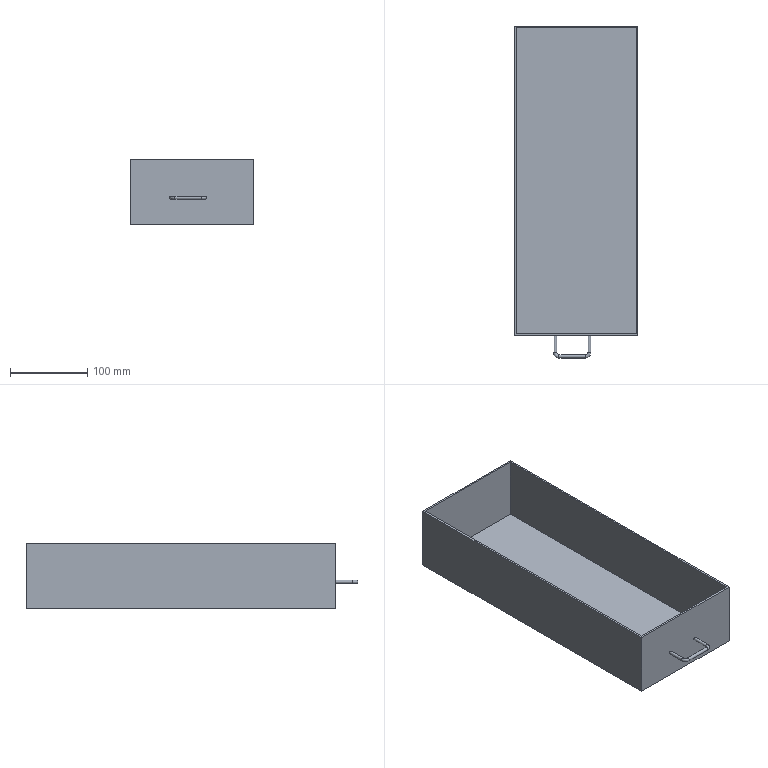Part | NX | features solid 2 | 1 solid | 16 faces | box 160 x 429 x 85 mm | volume 367407 mm3 | plane 11 | cylinder 3 | torus 2 | commonest cylinder face diameters 4 x3
STEP:
#1=CARTESIAN_POINT('',(363.,-305.,-247.));
#2=VERTEX_POINT('',#1);
#3=CARTESIAN_POINT('',(363.,-305.,-245.));
#4=DIRECTION('',(0.,-1.,0.));
#5=DIRECTION('',(0.,0.,-1.));
#6=AXIS2_PLACEMENT_3D('',#3,#4,#5);
#7=CIRCLE('',#6,2.);
#8=EDGE_CURVE('',#2,#2,#7,.F.);
#9=ORIENTED_EDGE('',*,*,#8,.T.);
#10=EDGE_LOOP('',(#9));
#11=FACE_BOUND('',#10,.T.);
#12=CARTESIAN_POINT('',(310.,-305.,-195.));
#13=VERTEX_POINT('',#12);
#14=CARTESIAN_POINT('',(470.,-305.,-195.));
#15=VERTEX_POINT('',#14);
#16=CARTESIAN_POINT('',(275.,-305.,-195.));
#17=DIRECTION('',(1.,0.,0.));
#18=VECTOR('',#17,1000.);
#19=LINE('',#16,#18);
#20=EDGE_CURVE('',#13,#15,#19,.T.);
#21=ORIENTED_EDGE('',*,*,#20,.F.);
#22=CARTESIAN_POINT('',(310.,-305.,-280.));
#23=VERTEX_POINT('',#22);
#24=CARTESIAN_POINT('',(310.,-305.,-145.));
#25=DIRECTION('',(0.,0.,-1.));
#26=VECTOR('',#25,1000.);
#27=LINE('',#24,#26);
#28=EDGE_CURVE('',#13,#23,#27,.T.);
#29=ORIENTED_EDGE('',*,*,#28,.T.);
#30=CARTESIAN_POINT('',(470.,-305.,-280.));
#31=VERTEX_POINT('',#30);
#32=CARTESIAN_POINT('',(275.,-305.,-280.));
#33=DIRECTION('',(1.,0.,0.));
#34=VECTOR('',#33,1000.);
#35=LINE('',#32,#34);
#36=EDGE_CURVE('',#23,#31,#35,.T.);
#37=ORIENTED_EDGE('',*,*,#36,.T.);
#38=CARTESIAN_POINT('',(470.,-305.,-145.));
#39=DIRECTION('',(0.,0.,1.));
#40=VECTOR('',#39,1000.);
#41=LINE('',#38,#40);
#42=EDGE_CURVE('',#15,#31,#41,.F.);
#43=ORIENTED_EDGE('',*,*,#42,.F.);
#44=EDGE_LOOP('',(#21,#29,#37,#43));
#45=FACE_BOUND('',#44,.T.);
#46=CARTESIAN_POINT('',(407.,-305.,-243.));
#47=VERTEX_POINT('',#46);
#48=CARTESIAN_POINT('',(407.,-305.,-245.));
#49=DIRECTION('',(0.,1.,0.));
#50=DIRECTION('',(0.,0.,1.));
#51=AXIS2_PLACEMENT_3D('',#48,#49,#50);
#52=CIRCLE('',#51,2.);
#53=EDGE_CURVE('',#47,#47,#52,.F.);
#54=ORIENTED_EDGE('',*,*,#53,.F.);
#55=EDGE_LOOP('',(#54));
#56=FACE_BOUND('',#55,.T.);
#57=CARTESIAN_POINT('',(275.,-305.,-145.));
#58=DIRECTION('',(0.,1.,0.));
#59=DIRECTION('',(0.,0.,1.));
#60=AXIS2_PLACEMENT_3D('',#57,#58,#59);
#61=PLANE('',#60);
#62=ADVANCED_FACE('',(#11,#45,#56),#61,.F.);
#63=CARTESIAN_POINT('',(470.,95.,-195.));
#64=VERTEX_POINT('',#63);
#65=CARTESIAN_POINT('',(470.,0.,-195.));
#66=DIRECTION('',(0.,-1.,0.));
#67=VECTOR('',#66,1000.);
#68=LINE('',#65,#67);
#69=EDGE_CURVE('',#15,#64,#68,.F.);
#70=ORIENTED_EDGE('',*,*,#69,.F.);
#71=ORIENTED_EDGE('',*,*,#42,.T.);
#72=CARTESIAN_POINT('',(470.,95.,-280.));
#73=VERTEX_POINT('',#72);
#74=CARTESIAN_POINT('',(470.,47.5,-280.));
#75=DIRECTION('',(0.,-1.,0.));
#76=VECTOR('',#75,1000.);
#77=LINE('',#74,#76);
#78=EDGE_CURVE('',#31,#73,#77,.F.);
#79=ORIENTED_EDGE('',*,*,#78,.T.);
#80=CARTESIAN_POINT('',(470.,95.,-125.));
#81=DIRECTION('',(0.,0.,-1.));
#82=VECTOR('',#81,1000.);
#83=LINE('',#80,#82);
#84=EDGE_CURVE('',#64,#73,#83,.T.);
#85=ORIENTED_EDGE('',*,*,#84,.F.);
#86=EDGE_LOOP('',(#70,#71,#79,#85));
#87=FACE_BOUND('',#86,.T.);
#88=CARTESIAN_POINT('',(470.,0.,-42.002));
#89=DIRECTION('',(-1.,0.,0.));
#90=DIRECTION('',(0.,0.,1.));
#91=AXIS2_PLACEMENT_3D('',#88,#89,#90);
#92=PLANE('',#91);
#93=ADVANCED_FACE('',(#87),#92,.F.);
#94=CARTESIAN_POINT('',(310.,95.,-195.));
#95=VERTEX_POINT('',#94);
#96=CARTESIAN_POINT('',(310.,-302.5,-195.));
#97=DIRECTION('',(0.,-1.,0.));
#98=VECTOR('',#97,1000.);
#99=LINE('',#96,#98);
#100=EDGE_CURVE('',#95,#13,#99,.T.);
#101=ORIENTED_EDGE('',*,*,#100,.F.);
#102=CARTESIAN_POINT('',(310.,95.,-280.));
#103=VERTEX_POINT('',#102);
#104=CARTESIAN_POINT('',(310.,95.,-125.));
#105=DIRECTION('',(0.,0.,1.));
#106=VECTOR('',#105,1000.);
#107=LINE('',#104,#106);
#108=EDGE_CURVE('',#95,#103,#107,.F.);
#109=ORIENTED_EDGE('',*,*,#108,.T.);
#110=CARTESIAN_POINT('',(310.,-302.5,-280.));
#111=DIRECTION('',(0.,-1.,0.));
#112=VECTOR('',#111,1000.);
#113=LINE('',#110,#112);
#114=EDGE_CURVE('',#103,#23,#113,.T.);
#115=ORIENTED_EDGE('',*,*,#114,.T.);
#116=ORIENTED_EDGE('',*,*,#28,.F.);
#117=EDGE_LOOP('',(#101,#109,#115,#116));
#118=FACE_BOUND('',#117,.T.);
#119=CARTESIAN_POINT('',(310.,-302.5,-145.));
#120=DIRECTION('',(1.,0.,0.));
#121=DIRECTION('',(0.,0.,-1.));
#122=AXIS2_PLACEMENT_3D('',#119,#120,#121);
#123=PLANE('',#122);
#124=ADVANCED_FACE('',(#118),#123,.F.);
#125=CARTESIAN_POINT('',(0.,95.,-195.));
#126=DIRECTION('',(1.,0.,0.));
#127=VECTOR('',#126,1000.);
#128=LINE('',#125,#127);
#129=EDGE_CURVE('',#64,#95,#128,.F.);
#130=ORIENTED_EDGE('',*,*,#129,.F.);
#131=ORIENTED_EDGE('',*,*,#84,.T.);
#132=CARTESIAN_POINT('',(492.5,95.,-280.));
#133=DIRECTION('',(1.,0.,0.));
#134=VECTOR('',#133,1000.);
#135=LINE('',#132,#134);
#136=EDGE_CURVE('',#73,#103,#135,.F.);
#137=ORIENTED_EDGE('',*,*,#136,.T.);
#138=ORIENTED_EDGE('',*,*,#108,.F.);
#139=EDGE_LOOP('',(#130,#131,#137,#138));
#140=FACE_BOUND('',#139,.T.);
#141=CARTESIAN_POINT('',(-640.,95.,-125.));
#142=DIRECTION('',(0.,-1.,0.));
#143=DIRECTION('',(1.,0.,0.));
#144=AXIS2_PLACEMENT_3D('',#141,#142,#143);
#145=PLANE('',#144);
#146=ADVANCED_FACE('',(#140),#145,.F.);
#147=ORIENTED_EDGE('',*,*,#136,.F.);
#148=ORIENTED_EDGE('',*,*,#78,.F.);
#149=ORIENTED_EDGE('',*,*,#36,.F.);
#150=ORIENTED_EDGE('',*,*,#114,.F.);
#151=EDGE_LOOP('',(#147,#148,#149,#150));
#152=FACE_BOUND('',#151,.T.);
#153=CARTESIAN_POINT('',(492.5,47.5,-280.));
#154=DIRECTION('',(0.,0.,1.));
#155=DIRECTION('',(1.,0.,0.));
#156=AXIS2_PLACEMENT_3D('',#153,#154,#155);
#157=PLANE('',#156);
#158=ADVANCED_FACE('',(#152),#157,.F.);
#159=CARTESIAN_POINT('',(468.,-302.5,-195.));
#160=VERTEX_POINT('',#159);
#161=CARTESIAN_POINT('',(312.5,-302.5,-195.));
#162=VERTEX_POINT('',#161);
#163=CARTESIAN_POINT('',(495.,-302.5,-195.));
#164=DIRECTION('',(-1.,0.,0.));
#165=VECTOR('',#164,1000.);
#166=LINE('',#163,#165);
#167=EDGE_CURVE('',#160,#162,#166,.T.);
#168=ORIENTED_EDGE('',*,*,#167,.T.);
#169=CARTESIAN_POINT('',(312.5,93.,-195.));
#170=VERTEX_POINT('',#169);
#171=CARTESIAN_POINT('',(312.5,-302.5,-195.));
#172=DIRECTION('',(0.,1.,0.));
#173=VECTOR('',#172,1000.);
#174=LINE('',#171,#173);
#175=EDGE_CURVE('',#162,#170,#174,.T.);
#176=ORIENTED_EDGE('',*,*,#175,.T.);
#177=CARTESIAN_POINT('',(468.,93.,-195.));
#178=VERTEX_POINT('',#177);
#179=CARTESIAN_POINT('',(275.,93.,-195.));
#180=DIRECTION('',(1.,0.,0.));
#181=VECTOR('',#180,1000.);
#182=LINE('',#179,#181);
#183=EDGE_CURVE('',#170,#178,#182,.T.);
#184=ORIENTED_EDGE('',*,*,#183,.T.);
#185=CARTESIAN_POINT('',(468.,47.5,-195.));
#186=DIRECTION('',(0.,-1.,0.));
#187=VECTOR('',#186,1000.);
#188=LINE('',#185,#187);
#189=EDGE_CURVE('',#178,#160,#188,.T.);
#190=ORIENTED_EDGE('',*,*,#189,.T.);
#191=EDGE_LOOP('',(#168,#176,#184,#190));
#192=FACE_BOUND('',#191,.T.);
#193=ORIENTED_EDGE('',*,*,#100,.T.);
#194=ORIENTED_EDGE('',*,*,#20,.T.);
#195=ORIENTED_EDGE('',*,*,#69,.T.);
#196=ORIENTED_EDGE('',*,*,#129,.T.);
#197=EDGE_LOOP('',(#193,#194,#195,#196));
#198=FACE_BOUND('',#197,.T.);
#199=CARTESIAN_POINT('',(0.,0.,-195.));
#200=DIRECTION('',(0.,0.,1.));
#201=DIRECTION('',(1.,0.,0.));
#202=AXIS2_PLACEMENT_3D('',#199,#200,#201);
#203=PLANE('',#202);
#204=ADVANCED_FACE('',(#192,#198),#203,.T.);
#205=CARTESIAN_POINT('',(468.,-302.5,-277.5));
#206=VERTEX_POINT('',#205);
#207=CARTESIAN_POINT('',(468.,93.,-277.5));
#208=VERTEX_POINT('',#207);
#209=CARTESIAN_POINT('',(468.,47.5,-277.5));
#210=DIRECTION('',(0.,1.,0.));
#211=VECTOR('',#210,1000.);
#212=LINE('',#209,#211);
#213=EDGE_CURVE('',#206,#208,#212,.T.);
#214=ORIENTED_EDGE('',*,*,#213,.T.);
#215=CARTESIAN_POINT('',(312.5,93.,-277.5));
#216=VERTEX_POINT('',#215);
#217=CARTESIAN_POINT('',(492.5,93.,-277.5));
#218=DIRECTION('',(-1.,0.,0.));
#219=VECTOR('',#218,1000.);
#220=LINE('',#217,#219);
#221=EDGE_CURVE('',#208,#216,#220,.T.);
#222=ORIENTED_EDGE('',*,*,#221,.T.);
#223=CARTESIAN_POINT('',(312.5,-302.5,-277.5));
#224=VERTEX_POINT('',#223);
#225=CARTESIAN_POINT('',(312.5,47.5,-277.5));
#226=DIRECTION('',(0.,-1.,0.));
#227=VECTOR('',#226,1000.);
#228=LINE('',#225,#227);
#229=EDGE_CURVE('',#216,#224,#228,.T.);
#230=ORIENTED_EDGE('',*,*,#229,.T.);
#231=CARTESIAN_POINT('',(277.5,-302.5,-277.5));
#232=DIRECTION('',(1.,0.,0.));
#233=VECTOR('',#232,1000.);
#234=LINE('',#231,#233);
#235=EDGE_CURVE('',#224,#206,#234,.T.);
#236=ORIENTED_EDGE('',*,*,#235,.T.);
#237=EDGE_LOOP('',(#214,#222,#230,#236));
#238=FACE_BOUND('',#237,.T.);
#239=CARTESIAN_POINT('',(492.5,47.5,-277.5));
#240=DIRECTION('',(0.,0.,1.));
#241=DIRECTION('',(1.,0.,0.));
#242=AXIS2_PLACEMENT_3D('',#239,#240,#241);
#243=PLANE('',#242);
#244=ADVANCED_FACE('',(#238),#243,.T.);
#245=ORIENTED_EDGE('',*,*,#189,.F.);
#246=CARTESIAN_POINT('',(468.,93.,-145.));
#247=DIRECTION('',(0.,0.,-1.));
#248=VECTOR('',#247,1000.);
#249=LINE('',#246,#248);
#250=EDGE_CURVE('',#178,#208,#249,.T.);
#251=ORIENTED_EDGE('',*,*,#250,.T.);
#252=ORIENTED_EDGE('',*,*,#213,.F.);
#253=CARTESIAN_POINT('',(468.,-302.5,-145.));
#254=DIRECTION('',(0.,0.,-1.));
#255=VECTOR('',#254,1000.);
#256=LINE('',#253,#255);
#257=EDGE_CURVE('',#160,#206,#256,.T.);
#258=ORIENTED_EDGE('',*,*,#257,.F.);
#259=EDGE_LOOP('',(#245,#251,#252,#258));
#260=FACE_BOUND('',#259,.T.);
#261=CARTESIAN_POINT('',(468.,47.5,-145.));
#262=DIRECTION('',(1.,0.,0.));
#263=DIRECTION('',(0.,0.,-1.));
#264=AXIS2_PLACEMENT_3D('',#261,#262,#263);
#265=PLANE('',#264);
#266=ADVANCED_FACE('',(#260),#265,.F.);
#267=ORIENTED_EDGE('',*,*,#175,.F.);
#268=CARTESIAN_POINT('',(312.5,-302.5,-145.));
#269=DIRECTION('',(0.,0.,-1.));
#270=VECTOR('',#269,1000.);
#271=LINE('',#268,#270);
#272=EDGE_CURVE('',#162,#224,#271,.T.);
#273=ORIENTED_EDGE('',*,*,#272,.T.);
#274=ORIENTED_EDGE('',*,*,#229,.F.);
#275=CARTESIAN_POINT('',(312.5,93.,-145.));
#276=DIRECTION('',(0.,0.,-1.));
#277=VECTOR('',#276,1000.);
#278=LINE('',#275,#277);
#279=EDGE_CURVE('',#170,#216,#278,.T.);
#280=ORIENTED_EDGE('',*,*,#279,.F.);
#281=EDGE_LOOP('',(#267,#273,#274,#280));
#282=FACE_BOUND('',#281,.T.);
#283=CARTESIAN_POINT('',(312.5,-302.5,-145.));
#284=DIRECTION('',(-1.,0.,0.));
#285=DIRECTION('',(0.,0.,1.));
#286=AXIS2_PLACEMENT_3D('',#283,#284,#285);
#287=PLANE('',#286);
#288=ADVANCED_FACE('',(#282),#287,.F.);
#289=ORIENTED_EDGE('',*,*,#183,.F.);
#290=ORIENTED_EDGE('',*,*,#279,.T.);
#291=ORIENTED_EDGE('',*,*,#221,.F.);
#292=ORIENTED_EDGE('',*,*,#250,.F.);
#293=EDGE_LOOP('',(#289,#290,#291,#292));
#294=FACE_BOUND('',#293,.T.);
#295=CARTESIAN_POINT('',(275.,93.,-145.));
#296=DIRECTION('',(0.,1.,0.));
#297=DIRECTION('',(0.,0.,1.));
#298=AXIS2_PLACEMENT_3D('',#295,#296,#297);
#299=PLANE('',#298);
#300=ADVANCED_FACE('',(#294),#299,.F.);
#301=ORIENTED_EDGE('',*,*,#167,.F.);
#302=ORIENTED_EDGE('',*,*,#257,.T.);
#303=ORIENTED_EDGE('',*,*,#235,.F.);
#304=ORIENTED_EDGE('',*,*,#272,.F.);
#305=EDGE_LOOP('',(#301,#302,#303,#304));
#306=FACE_BOUND('',#305,.T.);
#307=CARTESIAN_POINT('',(495.,-302.5,-145.));
#308=DIRECTION('',(0.,-1.,0.));
#309=DIRECTION('',(0.,0.,-1.));
#310=AXIS2_PLACEMENT_3D('',#307,#308,#309);
#311=PLANE('',#310);
#312=ADVANCED_FACE('',(#306),#311,.F.);
#313=CARTESIAN_POINT('',(368.,-332.,-247.));
#314=VERTEX_POINT('',#313);
#315=CARTESIAN_POINT('',(368.,-332.,-245.));
#316=DIRECTION('',(-1.,0.,0.));
#317=DIRECTION('',(0.,0.,-1.));
#318=AXIS2_PLACEMENT_3D('',#315,#316,#317);
#319=CIRCLE('',#318,2.);
#320=EDGE_CURVE('',#314,#314,#319,.T.);
#321=ORIENTED_EDGE('',*,*,#320,.T.);
#322=EDGE_LOOP('',(#321));
#323=FACE_BOUND('',#322,.T.);
#324=CARTESIAN_POINT('',(363.,-327.,-247.));
#325=VERTEX_POINT('',#324);
#326=CARTESIAN_POINT('',(363.,-327.,-245.));
#327=DIRECTION('',(0.,1.,0.));
#328=DIRECTION('',(0.,0.,-1.));
#329=AXIS2_PLACEMENT_3D('',#326,#327,#328);
#330=CIRCLE('',#329,2.);
#331=EDGE_CURVE('',#325,#325,#330,.T.);
#332=ORIENTED_EDGE('',*,*,#331,.F.);
#333=EDGE_LOOP('',(#332));
#334=FACE_BOUND('',#333,.T.);
#335=CARTESIAN_POINT('',(368.,-327.,-245.));
#336=DIRECTION('',(0.,0.,-1.));
#337=DIRECTION('',(-1.,0.,0.));
#338=AXIS2_PLACEMENT_3D('',#335,#336,#337);
#339=TOROIDAL_SURFACE('',#338,5.,2.);
#340=ADVANCED_FACE('',(#323,#334),#339,.T.);
#341=ORIENTED_EDGE('',*,*,#331,.T.);
#342=EDGE_LOOP('',(#341));
#343=FACE_BOUND('',#342,.T.);
#344=ORIENTED_EDGE('',*,*,#8,.F.);
#345=EDGE_LOOP('',(#344));
#346=FACE_BOUND('',#345,.T.);
#347=CARTESIAN_POINT('',(363.,-327.,-245.));
#348=DIRECTION('',(0.,1.,0.));
#349=DIRECTION('',(0.,0.,1.));
#350=AXIS2_PLACEMENT_3D('',#347,#348,#349);
#351=CYLINDRICAL_SURFACE('',#350,2.);
#352=ADVANCED_FACE('',(#343,#346),#351,.T.);
#353=CARTESIAN_POINT('',(402.,-332.,-247.));
#354=VERTEX_POINT('',#353);
#355=CARTESIAN_POINT('',(402.,-332.,-245.));
#356=DIRECTION('',(-1.,0.,0.));
#357=DIRECTION('',(0.,0.,-1.));
#358=AXIS2_PLACEMENT_3D('',#355,#356,#357);
#359=CIRCLE('',#358,2.);
#360=EDGE_CURVE('',#354,#354,#359,.T.);
#361=ORIENTED_EDGE('',*,*,#360,.T.);
#362=EDGE_LOOP('',(#361));
#363=FACE_BOUND('',#362,.T.);
#364=ORIENTED_EDGE('',*,*,#320,.F.);
#365=EDGE_LOOP('',(#364));
#366=FACE_BOUND('',#365,.T.);
#367=CARTESIAN_POINT('',(402.,-332.,-245.));
#368=DIRECTION('',(-1.,0.,0.));
#369=DIRECTION('',(0.,0.,1.));
#370=AXIS2_PLACEMENT_3D('',#367,#368,#369);
#371=CYLINDRICAL_SURFACE('',#370,2.);
#372=ADVANCED_FACE('',(#363,#366),#371,.T.);
#373=CARTESIAN_POINT('',(407.,-327.,-247.));
#374=VERTEX_POINT('',#373);
#375=CARTESIAN_POINT('',(407.,-327.,-245.));
#376=DIRECTION('',(0.,-1.,0.));
#377=DIRECTION('',(0.,0.,-1.));
#378=AXIS2_PLACEMENT_3D('',#375,#376,#377);
#379=CIRCLE('',#378,2.);
#380=EDGE_CURVE('',#374,#374,#379,.T.);
#381=ORIENTED_EDGE('',*,*,#380,.T.);
#382=EDGE_LOOP('',(#381));
#383=FACE_BOUND('',#382,.T.);
#384=ORIENTED_EDGE('',*,*,#360,.F.);
#385=EDGE_LOOP('',(#384));
#386=FACE_BOUND('',#385,.T.);
#387=CARTESIAN_POINT('',(402.,-327.,-245.));
#388=DIRECTION('',(0.,0.,-1.));
#389=DIRECTION('',(-1.,0.,0.));
#390=AXIS2_PLACEMENT_3D('',#387,#388,#389);
#391=TOROIDAL_SURFACE('',#390,5.,2.);
#392=ADVANCED_FACE('',(#383,#386),#391,.T.);
#393=ORIENTED_EDGE('',*,*,#380,.F.);
#394=EDGE_LOOP('',(#393));
#395=FACE_BOUND('',#394,.T.);
#396=ORIENTED_EDGE('',*,*,#53,.T.);
#397=EDGE_LOOP('',(#396));
#398=FACE_BOUND('',#397,.T.);
#399=CARTESIAN_POINT('',(407.,-327.,-245.));
#400=DIRECTION('',(0.,1.,0.));
#401=DIRECTION('',(0.,0.,1.));
#402=AXIS2_PLACEMENT_3D('',#399,#400,#401);
#403=CYLINDRICAL_SURFACE('',#402,2.);
#404=ADVANCED_FACE('',(#395,#398),#403,.T.);
#405=CLOSED_SHELL('',(#62,#93,#124,#146,#158,#204,#244,#266,#288,#300,#312,#340,#352,#372,#392,#404));
#406=MANIFOLD_SOLID_BREP('',#405);
#407=(LENGTH_UNIT()NAMED_UNIT(*)SI_UNIT(.MILLI.,.METRE.));
#408=UNCERTAINTY_MEASURE_WITH_UNIT(LENGTH_MEASURE(0.00001),#407,'','');
#409=(NAMED_UNIT(*)PLANE_ANGLE_UNIT()SI_UNIT($,.RADIAN.));
#410=(NAMED_UNIT(*)SI_UNIT($,.STERADIAN.)SOLID_ANGLE_UNIT());
#411=(GEOMETRIC_REPRESENTATION_CONTEXT(3)GLOBAL_UNCERTAINTY_ASSIGNED_CONTEXT((#408))GLOBAL_UNIT_ASSIGNED_CONTEXT((#407,#409,#410))REPRESENTATION_CONTEXT('',''));
#412=ADVANCED_BREP_SHAPE_REPRESENTATION('',(#406),#411);